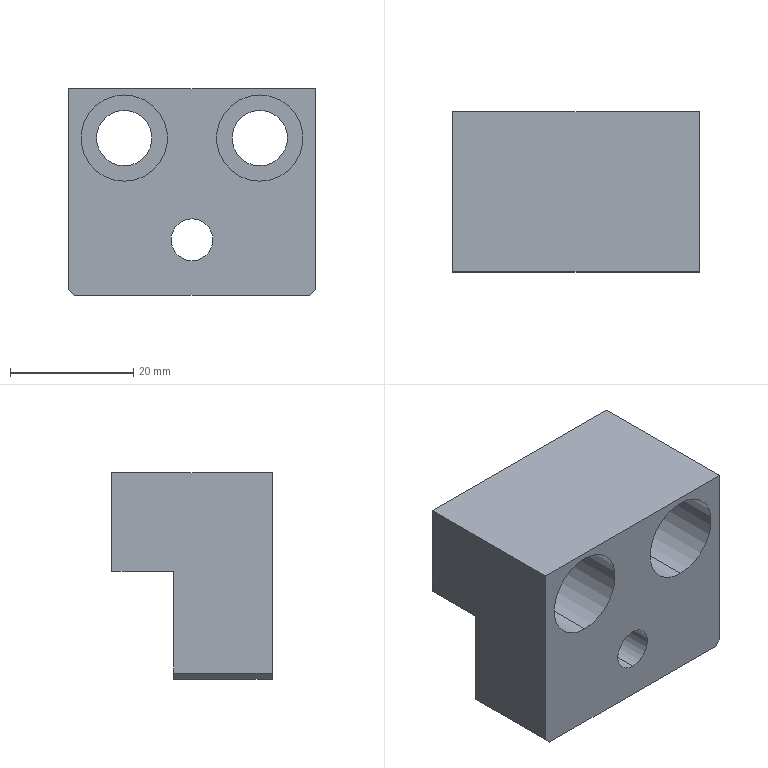Part | STEP file | PN_0015 Block_Default | 1 solid | 22 faces | box 40 x 26 x 33.5 mm | volume 22128 mm3 | plane 12 | cylinder 10 | commonest cylinder face diameters 9 x4 14 x4 6.8 x2